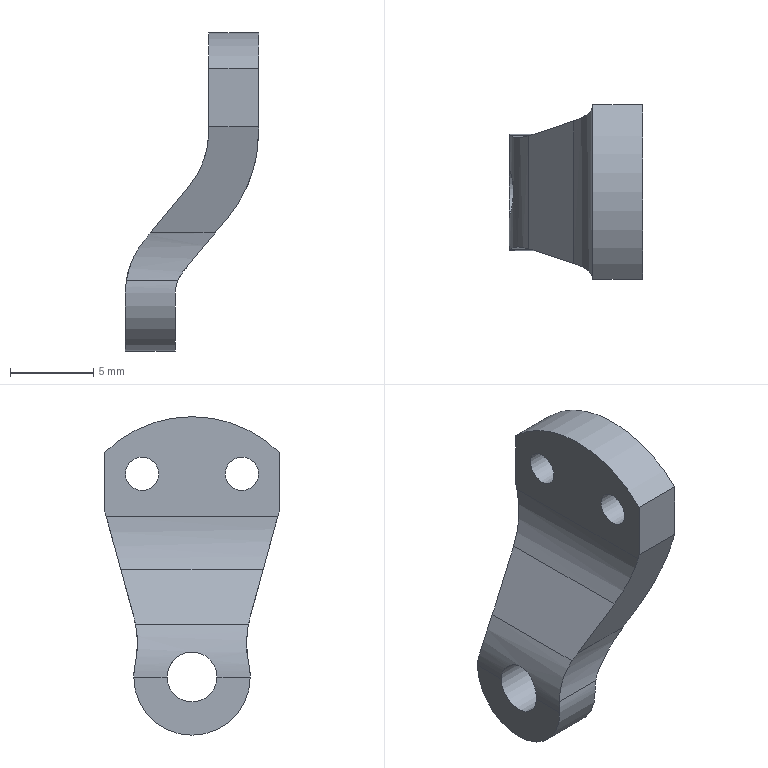Part | STEP file | 2-19 | 1 solid | 22 faces | box 8 x 10.503 x 19.146 mm | volume 448.562 mm3 | cylinder 12 | plane 10 | commonest cylinder face diameters 2 x2 4 x2 10 x2 12 x2 3 x1 7 x1